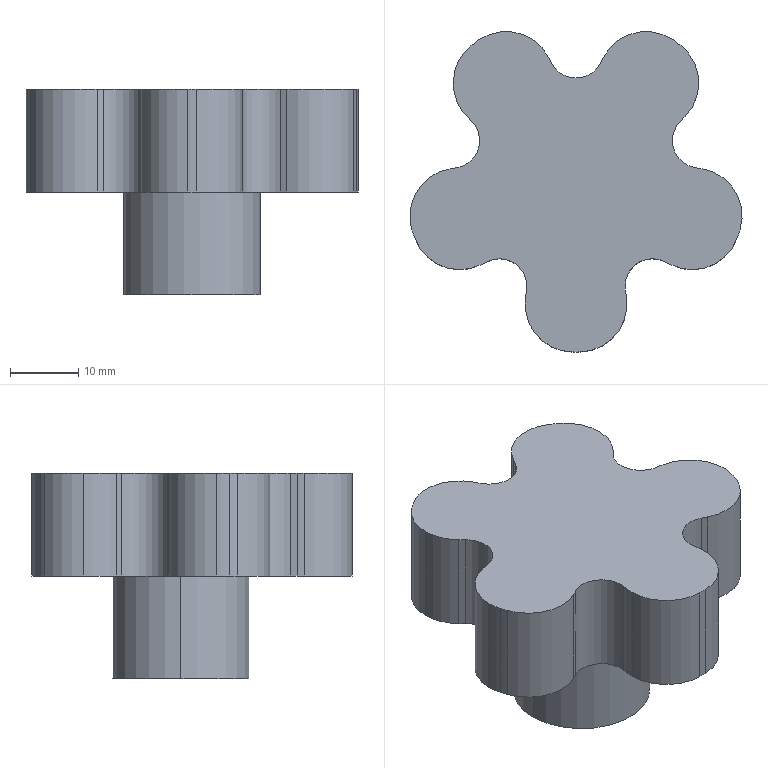Part | STEP file | Locking handwheel SGN-2-29 | 1 solid | 44 faces | box 48.498 x 46.815 x 30 mm | volume 24815 mm3 | cylinder 29 | plane 13 | cone 2 | commonest cylinder face diameters 14 x13 8 x7 50 x5 6.8 x2 20 x2